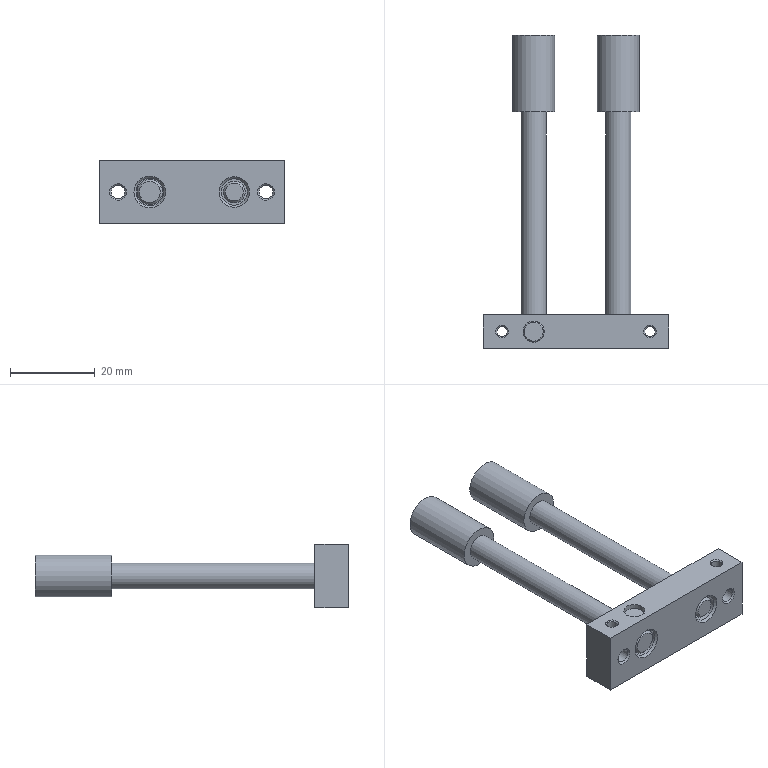Part | STEP file | ROTATION MC_NEW VER-0610_474 | 1 solid | 43 faces | box 44 x 74.1 x 15 mm | volume 10477 mm3 | plane 15 | cylinder 15 | cone 13 | commonest cylinder face diameters 2.459 x4 6 x3 3.242 x2 10 x2 5 x1 5.2 x1
STEP:
#1=CARTESIAN_POINT('',(223.531,700.368,-30.851));
#2=VERTEX_POINT('',#1);
#3=CARTESIAN_POINT('',(228.531,700.368,-30.851));
#4=DIRECTION('',(0.,1.,0.));
#5=DIRECTION('',(-1.,0.,0.));
#6=AXIS2_PLACEMENT_3D('',#3,#4,#5);
#7=CIRCLE('',#6,5.);
#8=EDGE_CURVE('',#2,#2,#7,.T.);
#9=ORIENTED_EDGE('',*,*,#8,.T.);
#10=EDGE_LOOP('',(#9));
#11=FACE_OUTER_BOUND('',#10,.T.);
#12=CARTESIAN_POINT('',(228.531,700.368,-25.851));
#13=DIRECTION('',(0.,-1.,0.));
#14=DIRECTION('',(0.,0.,-1.));
#15=AXIS2_PLACEMENT_3D('',#12,#13,#14);
#16=PLANE('',#15);
#17=ADVANCED_FACE('',(#11),#16,.F.);
#18=ORIENTED_EDGE('',*,*,#8,.F.);
#19=CARTESIAN_POINT('',(223.531,682.268,-30.851));
#20=VERTEX_POINT('',#19);
#21=CARTESIAN_POINT('',(223.531,700.368,-30.851));
#22=DIRECTION('',(0.,-1.,0.));
#23=VECTOR('',#22,5.);
#24=LINE('',#21,#23);
#25=EDGE_CURVE('',#2,#20,#24,.T.);
#26=ORIENTED_EDGE('',*,*,#25,.T.);
#27=CARTESIAN_POINT('',(228.531,682.268,-30.851));
#28=DIRECTION('',(0.,1.,0.));
#29=DIRECTION('',(-1.,0.,0.));
#30=AXIS2_PLACEMENT_3D('',#27,#28,#29);
#31=CIRCLE('',#30,5.);
#32=EDGE_CURVE('',#20,#20,#31,.T.);
#33=ORIENTED_EDGE('',*,*,#32,.T.);
#34=ORIENTED_EDGE('',*,*,#25,.F.);
#35=EDGE_LOOP('',(#18,#26,#33,#34));
#36=FACE_OUTER_BOUND('',#35,.T.);
#37=CARTESIAN_POINT('',(228.531,700.368,-30.851));
#38=DIRECTION('',(0.,1.,0.));
#39=DIRECTION('',(1.,0.,0.));
#40=AXIS2_PLACEMENT_3D('',#37,#38,#39);
#41=CYLINDRICAL_SURFACE('',#40,5.);
#42=ADVANCED_FACE('',(#36),#41,.T.);
#43=ORIENTED_EDGE('',*,*,#32,.F.);
#44=EDGE_LOOP('',(#43));
#45=FACE_OUTER_BOUND('',#44,.T.);
#46=CARTESIAN_POINT('',(225.531,682.268,-30.851));
#47=VERTEX_POINT('',#46);
#48=CARTESIAN_POINT('',(228.531,682.268,-30.851));
#49=DIRECTION('',(0.,1.,0.));
#50=DIRECTION('',(-1.,0.,0.));
#51=AXIS2_PLACEMENT_3D('',#48,#49,#50);
#52=CIRCLE('',#51,3.);
#53=EDGE_CURVE('',#47,#47,#52,.T.);
#54=ORIENTED_EDGE('',*,*,#53,.T.);
#55=EDGE_LOOP('',(#54));
#56=FACE_BOUND('',#55,.T.);
#57=CARTESIAN_POINT('',(228.531,682.268,-27.851));
#58=DIRECTION('',(0.,1.,0.));
#59=DIRECTION('',(0.,0.,1.));
#60=AXIS2_PLACEMENT_3D('',#57,#58,#59);
#61=PLANE('',#60);
#62=ADVANCED_FACE('',(#45,#56),#61,.F.);
#63=ORIENTED_EDGE('',*,*,#53,.F.);
#64=CARTESIAN_POINT('',(225.531,634.268,-30.851));
#65=VERTEX_POINT('',#64);
#66=CARTESIAN_POINT('',(225.531,700.368,-30.851));
#67=DIRECTION('',(0.,-1.,0.));
#68=VECTOR('',#67,3.);
#69=LINE('',#66,#68);
#70=EDGE_CURVE('',#47,#65,#69,.T.);
#71=ORIENTED_EDGE('',*,*,#70,.T.);
#72=CARTESIAN_POINT('',(228.531,634.268,-30.851));
#73=DIRECTION('',(0.,1.,0.));
#74=DIRECTION('',(-1.,0.,0.));
#75=AXIS2_PLACEMENT_3D('',#72,#73,#74);
#76=CIRCLE('',#75,3.);
#77=EDGE_CURVE('',#65,#65,#76,.T.);
#78=ORIENTED_EDGE('',*,*,#77,.T.);
#79=ORIENTED_EDGE('',*,*,#70,.F.);
#80=EDGE_LOOP('',(#63,#71,#78,#79));
#81=FACE_OUTER_BOUND('',#80,.T.);
#82=CARTESIAN_POINT('',(228.531,700.368,-30.851));
#83=DIRECTION('',(0.,1.,0.));
#84=DIRECTION('',(1.,0.,0.));
#85=AXIS2_PLACEMENT_3D('',#82,#83,#84);
#86=CYLINDRICAL_SURFACE('',#85,3.);
#87=ADVANCED_FACE('',(#81),#86,.T.);
#88=CARTESIAN_POINT('',(226.431,626.768,-30.851));
#89=VERTEX_POINT('',#88);
#90=CARTESIAN_POINT('',(228.531,626.768,-30.851));
#91=DIRECTION('',(0.,1.,0.));
#92=DIRECTION('',(-1.,0.,0.));
#93=AXIS2_PLACEMENT_3D('',#90,#91,#92);
#94=CIRCLE('',#93,2.1);
#95=EDGE_CURVE('',#89,#89,#94,.T.);
#96=ORIENTED_EDGE('',*,*,#95,.F.);
#97=EDGE_LOOP('',(#96));
#98=FACE_OUTER_BOUND('',#97,.T.);
#99=CARTESIAN_POINT('',(228.531,626.768,-28.751));
#100=DIRECTION('',(0.,-1.,0.));
#101=DIRECTION('',(0.,0.,-1.));
#102=AXIS2_PLACEMENT_3D('',#99,#100,#101);
#103=PLANE('',#102);
#104=ADVANCED_FACE('',(#98),#103,.T.);
#105=CARTESIAN_POINT('',(225.931,627.268,-30.851));
#106=VERTEX_POINT('',#105);
#107=CARTESIAN_POINT('',(228.531,627.268,-30.851));
#108=DIRECTION('',(0.,1.,0.));
#109=DIRECTION('',(-1.,0.,0.));
#110=AXIS2_PLACEMENT_3D('',#107,#108,#109);
#111=CIRCLE('',#110,2.6);
#112=EDGE_CURVE('',#106,#106,#111,.T.);
#113=ORIENTED_EDGE('',*,*,#112,.F.);
#114=CARTESIAN_POINT('',(225.931,627.268,-30.851));
#115=DIRECTION('',(0.7071,-0.7071,0.));
#116=VECTOR('',#115,2.6);
#117=LINE('',#114,#116);
#118=EDGE_CURVE('',#106,#89,#117,.T.);
#119=ORIENTED_EDGE('',*,*,#118,.T.);
#120=ORIENTED_EDGE('',*,*,#95,.T.);
#121=ORIENTED_EDGE('',*,*,#118,.F.);
#122=EDGE_LOOP('',(#113,#119,#120,#121));
#123=FACE_OUTER_BOUND('',#122,.T.);
#124=CARTESIAN_POINT('',(228.531,627.268,-30.851));
#125=DIRECTION('',(0.,1.,0.));
#126=DIRECTION('',(1.,0.,0.));
#127=AXIS2_PLACEMENT_3D('',#124,#125,#126);
#128=CONICAL_SURFACE('',#127,2.6,0.7854);
#129=ADVANCED_FACE('',(#123),#128,.T.);
#130=CARTESIAN_POINT('',(225.931,630.268,-30.851));
#131=VERTEX_POINT('',#130);
#132=CARTESIAN_POINT('',(228.531,630.268,-30.851));
#133=DIRECTION('',(0.,1.,0.));
#134=DIRECTION('',(-1.,0.,0.));
#135=AXIS2_PLACEMENT_3D('',#132,#133,#134);
#136=CIRCLE('',#135,2.6);
#137=EDGE_CURVE('',#131,#131,#136,.T.);
#138=ORIENTED_EDGE('',*,*,#137,.F.);
#139=CARTESIAN_POINT('',(225.931,630.268,-30.851));
#140=DIRECTION('',(0.,-1.,0.));
#141=VECTOR('',#140,2.6);
#142=LINE('',#139,#141);
#143=EDGE_CURVE('',#131,#106,#142,.T.);
#144=ORIENTED_EDGE('',*,*,#143,.T.);
#145=ORIENTED_EDGE('',*,*,#112,.T.);
#146=ORIENTED_EDGE('',*,*,#143,.F.);
#147=EDGE_LOOP('',(#138,#144,#145,#146));
#148=FACE_OUTER_BOUND('',#147,.T.);
#149=CARTESIAN_POINT('',(228.531,630.268,-30.851));
#150=DIRECTION('',(0.,1.,0.));
#151=DIRECTION('',(1.,0.,0.));
#152=AXIS2_PLACEMENT_3D('',#149,#150,#151);
#153=CYLINDRICAL_SURFACE('',#152,2.6);
#154=ADVANCED_FACE('',(#148),#153,.T.);
#155=CARTESIAN_POINT('',(225.431,630.268,-30.851));
#156=VERTEX_POINT('',#155);
#157=CARTESIAN_POINT('',(228.531,630.268,-30.851));
#158=DIRECTION('',(0.,1.,0.));
#159=DIRECTION('',(-1.,0.,0.));
#160=AXIS2_PLACEMENT_3D('',#157,#158,#159);
#161=CIRCLE('',#160,3.1);
#162=EDGE_CURVE('',#156,#156,#161,.T.);
#163=ORIENTED_EDGE('',*,*,#162,.F.);
#164=EDGE_LOOP('',(#163));
#165=FACE_OUTER_BOUND('',#164,.T.);
#166=ORIENTED_EDGE('',*,*,#137,.T.);
#167=EDGE_LOOP('',(#166));
#168=FACE_BOUND('',#167,.T.);
#169=CARTESIAN_POINT('',(228.531,630.268,-27.751));
#170=DIRECTION('',(0.,-1.,0.));
#171=DIRECTION('',(0.,0.,-1.));
#172=AXIS2_PLACEMENT_3D('',#169,#170,#171);
#173=PLANE('',#172);
#174=ADVANCED_FACE('',(#165,#168),#173,.T.);
#175=CARTESIAN_POINT('',(231.631,626.768,-30.851));
#176=VERTEX_POINT('',#175);
#177=CARTESIAN_POINT('',(225.431,626.768,-30.851));
#178=VERTEX_POINT('',#177);
#179=CARTESIAN_POINT('',(228.531,626.768,-30.851));
#180=DIRECTION('',(0.,1.,0.));
#181=DIRECTION('',(-1.,0.,0.));
#182=AXIS2_PLACEMENT_3D('',#179,#180,#181);
#183=CIRCLE('',#182,3.1);
#184=EDGE_CURVE('',#176,#178,#183,.T.);
#185=ORIENTED_EDGE('',*,*,#184,.F.);
#186=CARTESIAN_POINT('',(228.531,626.768,-30.851));
#187=DIRECTION('',(0.,1.,0.));
#188=DIRECTION('',(-1.,0.,0.));
#189=AXIS2_PLACEMENT_3D('',#186,#187,#188);
#190=CIRCLE('',#189,3.1);
#191=EDGE_CURVE('',#178,#176,#190,.T.);
#192=ORIENTED_EDGE('',*,*,#191,.F.);
#193=CARTESIAN_POINT('',(225.431,630.268,-30.851));
#194=DIRECTION('',(0.,1.,0.));
#195=VECTOR('',#194,3.1);
#196=LINE('',#193,#195);
#197=EDGE_CURVE('',#178,#156,#196,.T.);
#198=ORIENTED_EDGE('',*,*,#197,.T.);
#199=ORIENTED_EDGE('',*,*,#162,.T.);
#200=ORIENTED_EDGE('',*,*,#197,.F.);
#201=EDGE_LOOP('',(#185,#192,#198,#199,#200));
#202=FACE_OUTER_BOUND('',#201,.T.);
#203=CARTESIAN_POINT('',(228.531,630.268,-30.851));
#204=DIRECTION('',(0.,1.,0.));
#205=DIRECTION('',(1.,0.,0.));
#206=AXIS2_PLACEMENT_3D('',#203,#204,#205);
#207=CYLINDRICAL_SURFACE('',#206,3.1);
#208=ADVANCED_FACE('',(#202),#207,.F.);
#209=ORIENTED_EDGE('',*,*,#184,.T.);
#210=ORIENTED_EDGE('',*,*,#191,.T.);
#211=CARTESIAN_POINT('',(232.131,626.268,-30.851));
#212=VERTEX_POINT('',#211);
#213=CARTESIAN_POINT('',(232.131,626.268,-30.851));
#214=DIRECTION('',(0.7071,-0.7071,0.));
#215=VECTOR('',#214,3.6);
#216=LINE('',#213,#215);
#217=EDGE_CURVE('',#176,#212,#216,.T.);
#218=ORIENTED_EDGE('',*,*,#217,.T.);
#219=CARTESIAN_POINT('',(224.931,626.268,-30.851));
#220=VERTEX_POINT('',#219);
#221=CARTESIAN_POINT('',(228.531,626.268,-30.851));
#222=DIRECTION('',(0.,1.,0.));
#223=DIRECTION('',(-1.,0.,0.));
#224=AXIS2_PLACEMENT_3D('',#221,#222,#223);
#225=CIRCLE('',#224,3.6);
#226=EDGE_CURVE('',#220,#212,#225,.T.);
#227=ORIENTED_EDGE('',*,*,#226,.F.);
#228=CARTESIAN_POINT('',(228.531,626.268,-30.851));
#229=DIRECTION('',(0.,1.,0.));
#230=DIRECTION('',(-1.,0.,0.));
#231=AXIS2_PLACEMENT_3D('',#228,#229,#230);
#232=CIRCLE('',#231,3.6);
#233=EDGE_CURVE('',#212,#220,#232,.T.);
#234=ORIENTED_EDGE('',*,*,#233,.F.);
#235=ORIENTED_EDGE('',*,*,#217,.F.);
#236=EDGE_LOOP('',(#209,#210,#218,#227,#234,#235));
#237=FACE_OUTER_BOUND('',#236,.T.);
#238=CARTESIAN_POINT('',(228.531,626.268,-30.851));
#239=DIRECTION('',(0.,-1.,0.));
#240=DIRECTION('',(-1.,0.,0.));
#241=AXIS2_PLACEMENT_3D('',#238,#239,#240);
#242=CONICAL_SURFACE('',#241,3.6,0.7854);
#243=ADVANCED_FACE('',(#237),#242,.F.);
#244=CARTESIAN_POINT('',(206.281,630.268,-24.351));
#245=VERTEX_POINT('',#244);
#246=CARTESIAN_POINT('',(208.531,630.268,-24.351));
#247=DIRECTION('',(0.,0.,-1.));
#248=DIRECTION('',(-1.,0.,0.));
#249=AXIS2_PLACEMENT_3D('',#246,#247,#248);
#250=CIRCLE('',#249,2.25);
#251=EDGE_CURVE('',#245,#245,#250,.T.);
#252=ORIENTED_EDGE('',*,*,#251,.F.);
#253=EDGE_LOOP('',(#252));
#254=FACE_OUTER_BOUND('',#253,.T.);
#255=CARTESIAN_POINT('',(208.531,632.518,-24.351));
#256=DIRECTION('',(0.,0.,1.));
#257=DIRECTION('',(1.,0.,0.));
#258=AXIS2_PLACEMENT_3D('',#255,#256,#257);
#259=PLANE('',#258);
#260=ADVANCED_FACE('',(#254),#259,.T.);
#261=CARTESIAN_POINT('',(206.031,630.268,-24.601));
#262=VERTEX_POINT('',#261);
#263=CARTESIAN_POINT('',(208.531,630.268,-24.601));
#264=DIRECTION('',(0.,0.,-1.));
#265=DIRECTION('',(-1.,0.,0.));
#266=AXIS2_PLACEMENT_3D('',#263,#264,#265);
#267=CIRCLE('',#266,2.5);
#268=EDGE_CURVE('',#262,#262,#267,.T.);
#269=ORIENTED_EDGE('',*,*,#268,.F.);
#270=CARTESIAN_POINT('',(206.031,630.268,-24.601));
#271=DIRECTION('',(0.7071,0.,0.7071));
#272=VECTOR('',#271,2.5);
#273=LINE('',#270,#272);
#274=EDGE_CURVE('',#262,#245,#273,.T.);
#275=ORIENTED_EDGE('',*,*,#274,.T.);
#276=ORIENTED_EDGE('',*,*,#251,.T.);
#277=ORIENTED_EDGE('',*,*,#274,.F.);
#278=EDGE_LOOP('',(#269,#275,#276,#277));
#279=FACE_OUTER_BOUND('',#278,.T.);
#280=CARTESIAN_POINT('',(208.531,630.268,-24.601));
#281=DIRECTION('',(0.,0.,-1.));
#282=DIRECTION('',(1.,0.,0.));
#283=AXIS2_PLACEMENT_3D('',#280,#281,#282);
#284=CONICAL_SURFACE('',#283,2.5,0.7854);
#285=ADVANCED_FACE('',(#279),#284,.T.);
#286=CARTESIAN_POINT('',(206.031,630.268,-23.351));
#287=VERTEX_POINT('',#286);
#288=CARTESIAN_POINT('',(208.531,630.268,-23.351));
#289=DIRECTION('',(0.,0.,-1.));
#290=DIRECTION('',(-1.,0.,0.));
#291=AXIS2_PLACEMENT_3D('',#288,#289,#290);
#292=CIRCLE('',#291,2.5);
#293=EDGE_CURVE('',#287,#287,#292,.T.);
#294=ORIENTED_EDGE('',*,*,#293,.F.);
#295=CARTESIAN_POINT('',(206.031,630.268,-24.351));
#296=DIRECTION('',(0.,0.,-1.));
#297=VECTOR('',#296,2.5);
#298=LINE('',#295,#297);
#299=EDGE_CURVE('',#287,#262,#298,.T.);
#300=ORIENTED_EDGE('',*,*,#299,.T.);
#301=ORIENTED_EDGE('',*,*,#268,.T.);
#302=ORIENTED_EDGE('',*,*,#299,.F.);
#303=EDGE_LOOP('',(#294,#300,#301,#302));
#304=FACE_OUTER_BOUND('',#303,.T.);
#305=CARTESIAN_POINT('',(208.531,630.268,-24.351));
#306=DIRECTION('',(0.,0.,-1.));
#307=DIRECTION('',(1.,0.,0.));
#308=AXIS2_PLACEMENT_3D('',#305,#306,#307);
#309=CYLINDRICAL_SURFACE('',#308,2.5);
#310=ADVANCED_FACE('',(#304),#309,.F.);
#311=CARTESIAN_POINT('',(203.531,700.368,-30.851));
#312=VERTEX_POINT('',#311);
#313=CARTESIAN_POINT('',(208.531,700.368,-30.851));
#314=DIRECTION('',(0.,1.,0.));
#315=DIRECTION('',(-1.,0.,0.));
#316=AXIS2_PLACEMENT_3D('',#313,#314,#315);
#317=CIRCLE('',#316,5.);
#318=EDGE_CURVE('',#312,#312,#317,.T.);
#319=ORIENTED_EDGE('',*,*,#318,.T.);
#320=EDGE_LOOP('',(#319));
#321=FACE_OUTER_BOUND('',#320,.T.);
#322=CARTESIAN_POINT('',(208.531,700.368,-25.851));
#323=DIRECTION('',(0.,-1.,0.));
#324=DIRECTION('',(0.,0.,-1.));
#325=AXIS2_PLACEMENT_3D('',#322,#323,#324);
#326=PLANE('',#325);
#327=ADVANCED_FACE('',(#321),#326,.F.);
#328=ORIENTED_EDGE('',*,*,#318,.F.);
#329=CARTESIAN_POINT('',(203.531,682.268,-30.851));
#330=VERTEX_POINT('',#329);
#331=CARTESIAN_POINT('',(203.531,700.368,-30.851));
#332=DIRECTION('',(0.,-1.,0.));
#333=VECTOR('',#332,5.);
#334=LINE('',#331,#333);
#335=EDGE_CURVE('',#312,#330,#334,.T.);
#336=ORIENTED_EDGE('',*,*,#335,.T.);
#337=CARTESIAN_POINT('',(208.531,682.268,-30.851));
#338=DIRECTION('',(0.,1.,0.));
#339=DIRECTION('',(-1.,0.,0.));
#340=AXIS2_PLACEMENT_3D('',#337,#338,#339);
#341=CIRCLE('',#340,5.);
#342=EDGE_CURVE('',#330,#330,#341,.T.);
#343=ORIENTED_EDGE('',*,*,#342,.T.);
#344=ORIENTED_EDGE('',*,*,#335,.F.);
#345=EDGE_LOOP('',(#328,#336,#343,#344));
#346=FACE_OUTER_BOUND('',#345,.T.);
#347=CARTESIAN_POINT('',(208.531,700.368,-30.851));
#348=DIRECTION('',(0.,1.,0.));
#349=DIRECTION('',(1.,0.,0.));
#350=AXIS2_PLACEMENT_3D('',#347,#348,#349);
#351=CYLINDRICAL_SURFACE('',#350,5.);
#352=ADVANCED_FACE('',(#346),#351,.T.);
#353=ORIENTED_EDGE('',*,*,#342,.F.);
#354=EDGE_LOOP('',(#353));
#355=FACE_OUTER_BOUND('',#354,.T.);
#356=CARTESIAN_POINT('',(205.531,682.268,-30.851));
#357=VERTEX_POINT('',#356);
#358=CARTESIAN_POINT('',(208.531,682.268,-30.851));
#359=DIRECTION('',(0.,1.,0.));
#360=DIRECTION('',(-1.,0.,0.));
#361=AXIS2_PLACEMENT_3D('',#358,#359,#360);
#362=CIRCLE('',#361,3.);
#363=EDGE_CURVE('',#357,#357,#362,.T.);
#364=ORIENTED_EDGE('',*,*,#363,.T.);
#365=EDGE_LOOP('',(#364));
#366=FACE_BOUND('',#365,.T.);
#367=CARTESIAN_POINT('',(208.531,682.268,-27.851));
#368=DIRECTION('',(0.,1.,0.));
#369=DIRECTION('',(0.,0.,1.));
#370=AXIS2_PLACEMENT_3D('',#367,#368,#369);
#371=PLANE('',#370);
#372=ADVANCED_FACE('',(#355,#366),#371,.F.);
#373=ORIENTED_EDGE('',*,*,#363,.F.);
#374=CARTESIAN_POINT('',(205.531,634.268,-30.851));
#375=VERTEX_POINT('',#374);
#376=CARTESIAN_POINT('',(205.531,700.368,-30.851));
#377=DIRECTION('',(0.,-1.,0.));
#378=VECTOR('',#377,3.);
#379=LINE('',#376,#378);
#380=EDGE_CURVE('',#357,#375,#379,.T.);
#381=ORIENTED_EDGE('',*,*,#380,.T.);
#382=CARTESIAN_POINT('',(208.531,634.268,-30.851));
#383=DIRECTION('',(0.,1.,0.));
#384=DIRECTION('',(-1.,0.,0.));
#385=AXIS2_PLACEMENT_3D('',#382,#383,#384);
#386=CIRCLE('',#385,3.);
#387=EDGE_CURVE('',#375,#375,#386,.T.);
#388=ORIENTED_EDGE('',*,*,#387,.T.);
#389=ORIENTED_EDGE('',*,*,#380,.F.);
#390=EDGE_LOOP('',(#373,#381,#388,#389));
#391=FACE_OUTER_BOUND('',#390,.T.);
#392=CARTESIAN_POINT('',(208.531,700.368,-30.851));
#393=DIRECTION('',(0.,1.,0.));
#394=DIRECTION('',(1.,0.,0.));
#395=AXIS2_PLACEMENT_3D('',#392,#393,#394);
#396=CYLINDRICAL_SURFACE('',#395,3.);
#397=ADVANCED_FACE('',(#391),#396,.T.);
#398=CARTESIAN_POINT('',(206.031,626.768,-30.851));
#399=VERTEX_POINT('',#398);
#400=CARTESIAN_POINT('',(208.531,626.768,-30.851));
#401=DIRECTION('',(0.,1.,0.));
#402=DIRECTION('',(-1.,0.,0.));
#403=AXIS2_PLACEMENT_3D('',#400,#401,#402);
#404=CIRCLE('',#403,2.5);
#405=EDGE_CURVE('',#399,#399,#404,.T.);
#406=ORIENTED_EDGE('',*,*,#405,.F.);
#407=EDGE_LOOP('',(#406));
#408=FACE_OUTER_BOUND('',#407,.T.);
#409=CARTESIAN_POINT('',(208.531,626.768,-28.351));
#410=DIRECTION('',(0.,-1.,0.));
#411=DIRECTION('',(0.,0.,-1.));
#412=AXIS2_PLACEMENT_3D('',#409,#410,#411);
#413=PLANE('',#412);
#414=ADVANCED_FACE('',(#408),#413,.T.);
#415=CARTESIAN_POINT('',(205.531,627.268,-30.851));
#416=VERTEX_POINT('',#415);
#417=CARTESIAN_POINT('',(208.531,627.268,-30.851));
#418=DIRECTION('',(0.,1.,0.));
#419=DIRECTION('',(-1.,0.,0.));
#420=AXIS2_PLACEMENT_3D('',#417,#418,#419);
#421=CIRCLE('',#420,3.);
#422=EDGE_CURVE('',#416,#416,#421,.T.);
#423=ORIENTED_EDGE('',*,*,#422,.F.);
#424=CARTESIAN_POINT('',(205.531,627.268,-30.851));
#425=DIRECTION('',(0.7071,-0.7071,0.));
#426=VECTOR('',#425,3.);
#427=LINE('',#424,#426);
#428=EDGE_CURVE('',#416,#399,#427,.T.);
#429=ORIENTED_EDGE('',*,*,#428,.T.);
#430=ORIENTED_EDGE('',*,*,#405,.T.);
#431=ORIENTED_EDGE('',*,*,#428,.F.);
#432=EDGE_LOOP('',(#423,#429,#430,#431));
#433=FACE_OUTER_BOUND('',#432,.T.);
#434=CARTESIAN_POINT('',(208.531,627.268,-30.851));
#435=DIRECTION('',(0.,1.,0.));
#436=DIRECTION('',(1.,0.,0.));
#437=AXIS2_PLACEMENT_3D('',#434,#435,#436);
#438=CONICAL_SURFACE('',#437,3.,0.7854);
#439=ADVANCED_FACE('',(#433),#438,.T.);
#440=CARTESIAN_POINT('',(205.531,630.268,-30.851));
#441=VERTEX_POINT('',#440);
#442=CARTESIAN_POINT('',(208.531,630.268,-30.851));
#443=DIRECTION('',(0.,1.,0.));
#444=DIRECTION('',(-1.,0.,0.));
#445=AXIS2_PLACEMENT_3D('',#442,#443,#444);
#446=CIRCLE('',#445,3.);
#447=EDGE_CURVE('',#441,#441,#446,.T.);
#448=ORIENTED_EDGE('',*,*,#447,.F.);
#449=CARTESIAN_POINT('',(205.531,630.268,-30.851));
#450=DIRECTION('',(0.,-1.,0.));
#451=VECTOR('',#450,3.);
#452=LINE('',#449,#451);
#453=EDGE_CURVE('',#441,#416,#452,.T.);
#454=ORIENTED_EDGE('',*,*,#453,.T.);
#455=ORIENTED_EDGE('',*,*,#422,.T.);
#456=ORIENTED_EDGE('',*,*,#453,.F.);
#457=EDGE_LOOP('',(#448,#454,#455,#456));
#458=FACE_OUTER_BOUND('',#457,.T.);
#459=CARTESIAN_POINT('',(208.531,630.268,-30.851));
#460=DIRECTION('',(0.,1.,0.));
#461=DIRECTION('',(1.,0.,0.));
#462=AXIS2_PLACEMENT_3D('',#459,#460,#461);
#463=CYLINDRICAL_SURFACE('',#462,3.);
#464=ADVANCED_FACE('',(#458),#463,.T.);
#465=CARTESIAN_POINT('',(205.281,630.268,-30.851));
#466=VERTEX_POINT('',#465);
#467=CARTESIAN_POINT('',(208.531,630.268,-30.851));
#468=DIRECTION('',(0.,1.,0.));
#469=DIRECTION('',(-1.,0.,0.));
#470=AXIS2_PLACEMENT_3D('',#467,#468,#469);
#471=CIRCLE('',#470,3.25);
#472=EDGE_CURVE('',#466,#466,#471,.T.);
#473=ORIENTED_EDGE('',*,*,#472,.F.);
#474=EDGE_LOOP('',(#473));
#475=FACE_OUTER_BOUND('',#474,.T.);
#476=ORIENTED_EDGE('',*,*,#447,.T.);
#477=EDGE_LOOP('',(#476));
#478=FACE_BOUND('',#477,.T.);
#479=CARTESIAN_POINT('',(208.531,630.268,-27.601));
#480=DIRECTION('',(0.,-1.,0.));
#481=DIRECTION('',(0.,0.,-1.));
#482=AXIS2_PLACEMENT_3D('',#479,#480,#481);
#483=PLANE('',#482);
#484=ADVANCED_FACE('',(#475,#478),#483,.T.);
#485=CARTESIAN_POINT('',(211.781,626.768,-30.851));
#486=VERTEX_POINT('',#485);
#487=CARTESIAN_POINT('',(205.281,626.768,-30.851));
#488=VERTEX_POINT('',#487);
#489=CARTESIAN_POINT('',(208.531,626.768,-30.851));
#490=DIRECTION('',(0.,1.,0.));
#491=DIRECTION('',(-1.,0.,0.));
#492=AXIS2_PLACEMENT_3D('',#489,#490,#491);
#493=CIRCLE('',#492,3.25);
#494=EDGE_CURVE('',#486,#488,#493,.T.);
#495=ORIENTED_EDGE('',*,*,#494,.F.);
#496=CARTESIAN_POINT('',(208.531,626.768,-30.851));
#497=DIRECTION('',(0.,1.,0.));
#498=DIRECTION('',(-1.,0.,0.));
#499=AXIS2_PLACEMENT_3D('',#496,#497,#498);
#500=CIRCLE('',#499,3.25);
#501=EDGE_CURVE('',#488,#486,#500,.T.);
#502=ORIENTED_EDGE('',*,*,#501,.F.);
#503=CARTESIAN_POINT('',(205.281,630.268,-30.851));
#504=DIRECTION('',(0.,1.,0.));
#505=VECTOR('',#504,3.25);
#506=LINE('',#503,#505);
#507=EDGE_CURVE('',#488,#466,#506,.T.);
#508=ORIENTED_EDGE('',*,*,#507,.T.);
#509=ORIENTED_EDGE('',*,*,#472,.T.);
#510=ORIENTED_EDGE('',*,*,#507,.F.);
#511=EDGE_LOOP('',(#495,#502,#508,#509,#510));
#512=FACE_OUTER_BOUND('',#511,.T.);
#513=CARTESIAN_POINT('',(208.531,630.268,-30.851));
#514=DIRECTION('',(0.,1.,0.));
#515=DIRECTION('',(1.,0.,0.));
#516=AXIS2_PLACEMENT_3D('',#513,#514,#515);
#517=CYLINDRICAL_SURFACE('',#516,3.25);
#518=ADVANCED_FACE('',(#512),#517,.F.);
#519=ORIENTED_EDGE('',*,*,#494,.T.);
#520=ORIENTED_EDGE('',*,*,#501,.T.);
#521=CARTESIAN_POINT('',(212.281,626.268,-30.851));
#522=VERTEX_POINT('',#521);
#523=CARTESIAN_POINT('',(212.281,626.268,-30.851));
#524=DIRECTION('',(0.7071,-0.7071,0.));
#525=VECTOR('',#524,3.75);
#526=LINE('',#523,#525);
#527=EDGE_CURVE('',#486,#522,#526,.T.);
#528=ORIENTED_EDGE('',*,*,#527,.T.);
#529=CARTESIAN_POINT('',(204.781,626.268,-30.851));
#530=VERTEX_POINT('',#529);
#531=CARTESIAN_POINT('',(208.531,626.268,-30.851));
#532=DIRECTION('',(0.,1.,0.));
#533=DIRECTION('',(-1.,0.,0.));
#534=AXIS2_PLACEMENT_3D('',#531,#532,#533);
#535=CIRCLE('',#534,3.75);
#536=EDGE_CURVE('',#530,#522,#535,.T.);
#537=ORIENTED_EDGE('',*,*,#536,.F.);
#538=CARTESIAN_POINT('',(208.531,626.268,-30.851));
#539=DIRECTION('',(0.,1.,0.));
#540=DIRECTION('',(-1.,0.,0.));
#541=AXIS2_PLACEMENT_3D('',#538,#539,#540);
#542=CIRCLE('',#541,3.75);
#543=EDGE_CURVE('',#522,#530,#542,.T.);
#544=ORIENTED_EDGE('',*,*,#543,.F.);
#545=ORIENTED_EDGE('',*,*,#527,.F.);
#546=EDGE_LOOP('',(#519,#520,#528,#537,#544,#545));
#547=FACE_OUTER_BOUND('',#546,.T.);
#548=CARTESIAN_POINT('',(208.531,626.268,-30.851));
#549=DIRECTION('',(0.,-1.,0.));
#550=DIRECTION('',(-1.,0.,0.));
#551=AXIS2_PLACEMENT_3D('',#548,#549,#550);
#552=CONICAL_SURFACE('',#551,3.75,0.7854);
#553=ADVANCED_FACE('',(#547),#552,.F.);
#554=CARTESIAN_POINT('',(199.801,630.268,-23.622));
#555=VERTEX_POINT('',#554);
#556=CARTESIAN_POINT('',(202.26,630.268,-23.622));
#557=VERTEX_POINT('',#556);
#558=CARTESIAN_POINT('',(201.031,630.268,-23.622));
#559=DIRECTION('',(0.,0.,-1.));
#560=DIRECTION('',(-1.,0.,0.));
#561=AXIS2_PLACEMENT_3D('',#558,#559,#560);
#562=CIRCLE('',#561,1.23);
#563=EDGE_CURVE('',#555,#557,#562,.T.);
#564=ORIENTED_EDGE('',*,*,#563,.T.);
#565=CARTESIAN_POINT('',(202.531,630.268,-23.351));
#566=VERTEX_POINT('',#565);
#567=CARTESIAN_POINT('',(202.531,630.268,-23.351));
#568=DIRECTION('',(0.7071,0.,0.7071));
#569=VECTOR('',#568,1.5);
#570=LINE('',#567,#569);
#571=EDGE_CURVE('',#557,#566,#570,.T.);
#572=ORIENTED_EDGE('',*,*,#571,.T.);
#573=CARTESIAN_POINT('',(199.531,630.268,-23.351));
#574=VERTEX_POINT('',#573);
#575=CARTESIAN_POINT('',(201.031,630.268,-23.351));
#576=DIRECTION('',(0.,0.,-1.));
#577=DIRECTION('',(-1.,0.,0.));
#578=AXIS2_PLACEMENT_3D('',#575,#576,#577);
#579=CIRCLE('',#578,1.5);
#580=EDGE_CURVE('',#574,#566,#579,.T.);
#581=ORIENTED_EDGE('',*,*,#580,.F.);
#582=CARTESIAN_POINT('',(201.031,630.268,-23.351));
#583=DIRECTION('',(0.,0.,-1.));
#584=DIRECTION('',(-1.,0.,0.));
#585=AXIS2_PLACEMENT_3D('',#582,#583,#584);
#586=CIRCLE('',#585,1.5);
#587=EDGE_CURVE('',#566,#574,#586,.T.);
#588=ORIENTED_EDGE('',*,*,#587,.F.);
#589=ORIENTED_EDGE('',*,*,#571,.F.);
#590=CARTESIAN_POINT('',(201.031,630.268,-23.622));
#591=DIRECTION('',(0.,0.,-1.));
#592=DIRECTION('',(-1.,0.,0.));
#593=AXIS2_PLACEMENT_3D('',#590,#591,#592);
#594=CIRCLE('',#593,1.23);
#595=EDGE_CURVE('',#557,#555,#594,.T.);
#596=ORIENTED_EDGE('',*,*,#595,.T.);
#597=EDGE_LOOP('',(#564,#572,#581,#588,#589,#596));
#598=FACE_OUTER_BOUND('',#597,.T.);
#599=CARTESIAN_POINT('',(201.031,630.268,-23.351));
#600=DIRECTION('',(0.,0.,1.));
#601=DIRECTION('',(-1.,0.,0.));
#602=AXIS2_PLACEMENT_3D('',#599,#600,#601);
#603=CONICAL_SURFACE('',#602,1.5,0.7854);
#604=ADVANCED_FACE('',(#598),#603,.F.);
#605=ORIENTED_EDGE('',*,*,#563,.F.);
#606=CARTESIAN_POINT('',(199.801,630.268,-29.795));
#607=VERTEX_POINT('',#606);
#608=CARTESIAN_POINT('',(199.801,630.268,-38.351));
#609=DIRECTION('',(0.,0.,-1.));
#610=VECTOR('',#609,1.23);
#611=LINE('',#608,#610);
#612=EDGE_CURVE('',#555,#607,#611,.T.);
#613=ORIENTED_EDGE('',*,*,#612,.T.);
#614=CARTESIAN_POINT('',(199.801,630.268,-29.795));
#615=CARTESIAN_POINT('',(199.801,630.186,-29.795));
#616=CARTESIAN_POINT('',(199.81,630.103,-29.785));
#617=CARTESIAN_POINT('',(199.843,629.941,-29.748));
#618=CARTESIAN_POINT('',(199.867,629.863,-29.722));
#619=CARTESIAN_POINT('',(199.962,629.639,-29.629));
#620=CARTESIAN_POINT('',(200.055,629.506,-29.551));
#621=CARTESIAN_POINT('',(200.266,629.295,-29.417));
#622=CARTESIAN_POINT('',(200.399,629.201,-29.35));
#623=CARTESIAN_POINT('',(200.701,629.073,-29.256));
#624=CARTESIAN_POINT('',(200.869,629.039,-29.23));
#625=CARTESIAN_POINT('',(201.193,629.039,-29.23));
#626=CARTESIAN_POINT('',(201.361,629.073,-29.256));
#627=CARTESIAN_POINT('',(201.662,629.201,-29.35));
#628=CARTESIAN_POINT('',(201.796,629.295,-29.417));
#629=CARTESIAN_POINT('',(202.007,629.506,-29.551));
#630=CARTESIAN_POINT('',(202.099,629.639,-29.629));
#631=CARTESIAN_POINT('',(202.194,629.863,-29.722));
#632=CARTESIAN_POINT('',(202.219,629.941,-29.748));
#633=CARTESIAN_POINT('',(202.252,630.103,-29.785));
#634=CARTESIAN_POINT('',(202.26,630.186,-29.795));
#635=CARTESIAN_POINT('',(202.26,630.351,-29.795));
#636=CARTESIAN_POINT('',(202.252,630.434,-29.785));
#637=CARTESIAN_POINT('',(202.219,630.596,-29.748));
#638=CARTESIAN_POINT('',(202.194,630.674,-29.722));
#639=CARTESIAN_POINT('',(202.099,630.898,-29.629));
#640=CARTESIAN_POINT('',(202.007,631.031,-29.551));
#641=CARTESIAN_POINT('',(201.796,631.242,-29.417));
#642=CARTESIAN_POINT('',(201.662,631.336,-29.35));
#643=CARTESIAN_POINT('',(201.361,631.464,-29.256));
#644=CARTESIAN_POINT('',(201.193,631.498,-29.23));
#645=CARTESIAN_POINT('',(200.869,631.498,-29.23));
#646=CARTESIAN_POINT('',(200.701,631.464,-29.256));
#647=CARTESIAN_POINT('',(200.399,631.336,-29.35));
#648=CARTESIAN_POINT('',(200.266,631.242,-29.417));
#649=CARTESIAN_POINT('',(200.055,631.031,-29.551));
#650=CARTESIAN_POINT('',(199.962,630.898,-29.629));
#651=CARTESIAN_POINT('',(199.867,630.674,-29.722));
#652=CARTESIAN_POINT('',(199.843,630.596,-29.748));
#653=CARTESIAN_POINT('',(199.81,630.434,-29.785));
#654=CARTESIAN_POINT('',(199.801,630.351,-29.795));
#655=CARTESIAN_POINT('',(199.801,630.268,-29.795));
#656=B_SPLINE_CURVE_WITH_KNOTS('',3,(#614,#615,#616,#617,#618,#619,#620,#621,#622,#623,#624,#625,#626,#627,#628,#629,#630,#631,#632,#633,#634,#635,#636,#637,#638,#639,#640,#641,#642,#643,#644,#645,#646,#647,#648,#649,#650,#651,#652,#653,#654,#655),.UNSPECIFIED.,.T.,.F.,(4,2,2,2,2,2,2,2,2,2,2,2,2,2,2,2,2,2,2,2,4),(-0.7858,-0.7609,-0.7361,-0.6864,-0.6379,-0.5893,-0.5408,-0.4922,-0.4426,-0.4177,-0.3929,-0.3681,-0.3432,-0.2935,-0.245,-0.1964,-0.1479,-0.09934,-0.04967,-0.02483,0.),.UNSPECIFIED.);
#657=EDGE_CURVE('',#607,#607,#656,.T.);
#658=ORIENTED_EDGE('',*,*,#657,.F.);
#659=ORIENTED_EDGE('',*,*,#612,.F.);
#660=ORIENTED_EDGE('',*,*,#595,.F.);
#661=EDGE_LOOP('',(#605,#613,#658,#659,#660));
#662=FACE_OUTER_BOUND('',#661,.T.);
#663=CARTESIAN_POINT('',(201.031,630.268,-38.351));
#664=DIRECTION('',(0.,0.,-1.));
#665=DIRECTION('',(1.,0.,0.));
#666=AXIS2_PLACEMENT_3D('',#663,#664,#665);
#667=CYLINDRICAL_SURFACE('',#666,1.23);
#668=ADVANCED_FACE('',(#662),#667,.F.);
#669=CARTESIAN_POINT('',(199.801,630.268,-38.081));
#670=VERTEX_POINT('',#669);
#671=CARTESIAN_POINT('',(201.031,630.268,-38.081));
#672=DIRECTION('',(0.,0.,-1.));
#673=DIRECTION('',(-1.,0.,0.));
#674=AXIS2_PLACEMENT_3D('',#671,#672,#673);
#675=CIRCLE('',#674,1.23);
#676=EDGE_CURVE('',#670,#670,#675,.T.);
#677=ORIENTED_EDGE('',*,*,#676,.F.);
#678=CARTESIAN_POINT('',(199.531,630.268,-38.351));
#679=VERTEX_POINT('',#678);
#680=CARTESIAN_POINT('',(199.801,630.268,-38.081));
#681=DIRECTION('',(-0.7071,0.,-0.7071));
#682=VECTOR('',#681,1.23);
#683=LINE('',#680,#682);
#684=EDGE_CURVE('',#670,#679,#683,.T.);
#685=ORIENTED_EDGE('',*,*,#684,.T.);
#686=CARTESIAN_POINT('',(201.031,630.268,-38.351));
#687=DIRECTION('',(0.,0.,-1.));
#688=DIRECTION('',(-1.,0.,0.));
#689=AXIS2_PLACEMENT_3D('',#686,#687,#688);
#690=CIRCLE('',#689,1.5);
#691=EDGE_CURVE('',#679,#679,#690,.T.);
#692=ORIENTED_EDGE('',*,*,#691,.T.);
#693=ORIENTED_EDGE('',*,*,#684,.F.);
#694=EDGE_LOOP('',(#677,#685,#692,#693));
#695=FACE_OUTER_BOUND('',#694,.T.);
#696=CARTESIAN_POINT('',(201.031,630.268,-38.081));
#697=DIRECTION('',(0.,0.,-1.));
#698=DIRECTION('',(1.,0.,0.));
#699=AXIS2_PLACEMENT_3D('',#696,#697,#698);
#700=CONICAL_SURFACE('',#699,1.23,0.7854);
#701=ADVANCED_FACE('',(#695),#700,.F.);
#702=CARTESIAN_POINT('',(199.801,630.268,-31.908));
#703=VERTEX_POINT('',#702);
#704=CARTESIAN_POINT('',(199.801,630.268,-31.908));
#705=CARTESIAN_POINT('',(199.801,630.351,-31.908));
#706=CARTESIAN_POINT('',(199.81,630.434,-31.918));
#707=CARTESIAN_POINT('',(199.843,630.596,-31.954));
#708=CARTESIAN_POINT('',(199.867,630.674,-31.981));
#709=CARTESIAN_POINT('',(199.962,630.898,-32.073));
#710=CARTESIAN_POINT('',(200.055,631.031,-32.152));
#711=CARTESIAN_POINT('',(200.266,631.242,-32.286));
#712=CARTESIAN_POINT('',(200.399,631.336,-32.353));
#713=CARTESIAN_POINT('',(200.701,631.464,-32.446));
#714=CARTESIAN_POINT('',(200.869,631.498,-32.472));
#715=CARTESIAN_POINT('',(201.193,631.498,-32.472));
#716=CARTESIAN_POINT('',(201.361,631.464,-32.446));
#717=CARTESIAN_POINT('',(201.662,631.336,-32.353));
#718=CARTESIAN_POINT('',(201.796,631.242,-32.286));
#719=CARTESIAN_POINT('',(202.007,631.031,-32.152));
#720=CARTESIAN_POINT('',(202.099,630.898,-32.073));
#721=CARTESIAN_POINT('',(202.194,630.674,-31.981));
#722=CARTESIAN_POINT('',(202.219,630.596,-31.954));
#723=CARTESIAN_POINT('',(202.252,630.434,-31.918));
#724=CARTESIAN_POINT('',(202.26,630.351,-31.908));
#725=CARTESIAN_POINT('',(202.26,630.186,-31.908));
#726=CARTESIAN_POINT('',(202.252,630.103,-31.918));
#727=CARTESIAN_POINT('',(202.219,629.941,-31.954));
#728=CARTESIAN_POINT('',(202.194,629.863,-31.981));
#729=CARTESIAN_POINT('',(202.099,629.639,-32.073));
#730=CARTESIAN_POINT('',(202.007,629.506,-32.152));
#731=CARTESIAN_POINT('',(201.796,629.295,-32.286));
#732=CARTESIAN_POINT('',(201.662,629.201,-32.353));
#733=CARTESIAN_POINT('',(201.361,629.073,-32.446));
#734=CARTESIAN_POINT('',(201.193,629.039,-32.472));
#735=CARTESIAN_POINT('',(200.869,629.039,-32.472));
#736=CARTESIAN_POINT('',(200.701,629.073,-32.446));
#737=CARTESIAN_POINT('',(200.399,629.201,-32.353));
#738=CARTESIAN_POINT('',(200.266,629.295,-32.286));
#739=CARTESIAN_POINT('',(200.055,629.506,-32.152));
#740=CARTESIAN_POINT('',(199.962,629.639,-32.073));
#741=CARTESIAN_POINT('',(199.867,629.863,-31.981));
#742=CARTESIAN_POINT('',(199.843,629.941,-31.954));
#743=CARTESIAN_POINT('',(199.81,630.103,-31.918));
#744=CARTESIAN_POINT('',(199.801,630.186,-31.908));
#745=CARTESIAN_POINT('',(199.801,630.268,-31.908));
#746=B_SPLINE_CURVE_WITH_KNOTS('',3,(#704,#705,#706,#707,#708,#709,#710,#711,#712,#713,#714,#715,#716,#717,#718,#719,#720,#721,#722,#723,#724,#725,#726,#727,#728,#729,#730,#731,#732,#733,#734,#735,#736,#737,#738,#739,#740,#741,#742,#743,#744,#745),.UNSPECIFIED.,.T.,.F.,(4,2,2,2,2,2,2,2,2,2,2,2,2,2,2,2,2,2,2,2,4),(-0.7858,-0.7609,-0.7361,-0.6864,-0.6379,-0.5893,-0.5408,-0.4922,-0.4426,-0.4177,-0.3929,-0.3681,-0.3432,-0.2935,-0.245,-0.1964,-0.1479,-0.09934,-0.04967,-0.02483,0.),.UNSPECIFIED.);
#747=EDGE_CURVE('',#703,#703,#746,.T.);
#748=ORIENTED_EDGE('',*,*,#747,.F.);
#749=CARTESIAN_POINT('',(199.801,630.268,-38.351));
#750=DIRECTION('',(0.,0.,-1.));
#751=VECTOR('',#750,1.23);
#752=LINE('',#749,#751);
#753=EDGE_CURVE('',#703,#670,#752,.T.);
#754=ORIENTED_EDGE('',*,*,#753,.T.);
#755=ORIENTED_EDGE('',*,*,#676,.T.);
#756=ORIENTED_EDGE('',*,*,#753,.F.);
#757=EDGE_LOOP('',(#748,#754,#755,#756));
#758=FACE_OUTER_BOUND('',#757,.T.);
#759=CARTESIAN_POINT('',(201.031,630.268,-38.351));
#760=DIRECTION('',(0.,0.,-1.));
#761=DIRECTION('',(1.,0.,0.));
#762=AXIS2_PLACEMENT_3D('',#759,#760,#761);
#763=CYLINDRICAL_SURFACE('',#762,1.23);
#764=ADVANCED_FACE('',(#758),#763,.F.);
#765=CARTESIAN_POINT('',(234.801,630.268,-23.622));
#766=VERTEX_POINT('',#765);
#767=CARTESIAN_POINT('',(237.26,630.268,-23.622));
#768=VERTEX_POINT('',#767);
#769=CARTESIAN_POINT('',(236.031,630.268,-23.622));
#770=DIRECTION('',(0.,0.,-1.));
#771=DIRECTION('',(-1.,0.,0.));
#772=AXIS2_PLACEMENT_3D('',#769,#770,#771);
#773=CIRCLE('',#772,1.23);
#774=EDGE_CURVE('',#766,#768,#773,.T.);
#775=ORIENTED_EDGE('',*,*,#774,.T.);
#776=CARTESIAN_POINT('',(237.531,630.268,-23.351));
#777=VERTEX_POINT('',#776);
#778=CARTESIAN_POINT('',(237.531,630.268,-23.351));
#779=DIRECTION('',(0.7071,0.,0.7071));
#780=VECTOR('',#779,1.5);
#781=LINE('',#778,#780);
#782=EDGE_CURVE('',#768,#777,#781,.T.);
#783=ORIENTED_EDGE('',*,*,#782,.T.);
#784=CARTESIAN_POINT('',(234.531,630.268,-23.351));
#785=VERTEX_POINT('',#784);
#786=CARTESIAN_POINT('',(236.031,630.268,-23.351));
#787=DIRECTION('',(0.,0.,-1.));
#788=DIRECTION('',(-1.,0.,0.));
#789=AXIS2_PLACEMENT_3D('',#786,#787,#788);
#790=CIRCLE('',#789,1.5);
#791=EDGE_CURVE('',#785,#777,#790,.T.);
#792=ORIENTED_EDGE('',*,*,#791,.F.);
#793=CARTESIAN_POINT('',(236.031,630.268,-23.351));
#794=DIRECTION('',(0.,0.,-1.));
#795=DIRECTION('',(-1.,0.,0.));
#796=AXIS2_PLACEMENT_3D('',#793,#794,#795);
#797=CIRCLE('',#796,1.5);
#798=EDGE_CURVE('',#777,#785,#797,.T.);
#799=ORIENTED_EDGE('',*,*,#798,.F.);
#800=ORIENTED_EDGE('',*,*,#782,.F.);
#801=CARTESIAN_POINT('',(236.031,630.268,-23.622));
#802=DIRECTION('',(0.,0.,-1.));
#803=DIRECTION('',(-1.,0.,0.));
#804=AXIS2_PLACEMENT_3D('',#801,#802,#803);
#805=CIRCLE('',#804,1.23);
#806=EDGE_CURVE('',#768,#766,#805,.T.);
#807=ORIENTED_EDGE('',*,*,#806,.T.);
#808=EDGE_LOOP('',(#775,#783,#792,#799,#800,#807));
#809=FACE_OUTER_BOUND('',#808,.T.);
#810=CARTESIAN_POINT('',(236.031,630.268,-23.351));
#811=DIRECTION('',(0.,0.,1.));
#812=DIRECTION('',(-1.,0.,0.));
#813=AXIS2_PLACEMENT_3D('',#810,#811,#812);
#814=CONICAL_SURFACE('',#813,1.5,0.7854);
#815=ADVANCED_FACE('',(#809),#814,.F.);
#816=ORIENTED_EDGE('',*,*,#774,.F.);
#817=CARTESIAN_POINT('',(234.801,630.268,-29.795));
#818=VERTEX_POINT('',#817);
#819=CARTESIAN_POINT('',(234.801,630.268,-38.351));
#820=DIRECTION('',(0.,0.,-1.));
#821=VECTOR('',#820,1.23);
#822=LINE('',#819,#821);
#823=EDGE_CURVE('',#766,#818,#822,.T.);
#824=ORIENTED_EDGE('',*,*,#823,.T.);
#825=CARTESIAN_POINT('',(234.801,630.268,-29.795));
#826=CARTESIAN_POINT('',(234.801,630.186,-29.795));
#827=CARTESIAN_POINT('',(234.81,630.103,-29.785));
#828=CARTESIAN_POINT('',(234.843,629.941,-29.748));
#829=CARTESIAN_POINT('',(234.867,629.863,-29.722));
#830=CARTESIAN_POINT('',(234.962,629.639,-29.629));
#831=CARTESIAN_POINT('',(235.055,629.506,-29.551));
#832=CARTESIAN_POINT('',(235.266,629.295,-29.417));
#833=CARTESIAN_POINT('',(235.399,629.201,-29.35));
#834=CARTESIAN_POINT('',(235.701,629.073,-29.256));
#835=CARTESIAN_POINT('',(235.869,629.039,-29.23));
#836=CARTESIAN_POINT('',(236.193,629.039,-29.23));
#837=CARTESIAN_POINT('',(236.361,629.073,-29.256));
#838=CARTESIAN_POINT('',(236.662,629.201,-29.35));
#839=CARTESIAN_POINT('',(236.796,629.295,-29.417));
#840=CARTESIAN_POINT('',(237.007,629.506,-29.551));
#841=CARTESIAN_POINT('',(237.099,629.639,-29.629));
#842=CARTESIAN_POINT('',(237.194,629.863,-29.722));
#843=CARTESIAN_POINT('',(237.219,629.941,-29.748));
#844=CARTESIAN_POINT('',(237.252,630.103,-29.785));
#845=CARTESIAN_POINT('',(237.26,630.186,-29.795));
#846=CARTESIAN_POINT('',(237.26,630.351,-29.795));
#847=CARTESIAN_POINT('',(237.252,630.434,-29.785));
#848=CARTESIAN_POINT('',(237.219,630.596,-29.748));
#849=CARTESIAN_POINT('',(237.194,630.674,-29.722));
#850=CARTESIAN_POINT('',(237.099,630.898,-29.629));
#851=CARTESIAN_POINT('',(237.007,631.031,-29.551));
#852=CARTESIAN_POINT('',(236.796,631.242,-29.417));
#853=CARTESIAN_POINT('',(236.662,631.336,-29.35));
#854=CARTESIAN_POINT('',(236.361,631.464,-29.256));
#855=CARTESIAN_POINT('',(236.193,631.498,-29.23));
#856=CARTESIAN_POINT('',(235.869,631.498,-29.23));
#857=CARTESIAN_POINT('',(235.701,631.464,-29.256));
#858=CARTESIAN_POINT('',(235.399,631.336,-29.35));
#859=CARTESIAN_POINT('',(235.266,631.242,-29.417));
#860=CARTESIAN_POINT('',(235.055,631.031,-29.551));
#861=CARTESIAN_POINT('',(234.962,630.898,-29.629));
#862=CARTESIAN_POINT('',(234.867,630.674,-29.722));
#863=CARTESIAN_POINT('',(234.843,630.596,-29.748));
#864=CARTESIAN_POINT('',(234.81,630.434,-29.785));
#865=CARTESIAN_POINT('',(234.801,630.351,-29.795));
#866=CARTESIAN_POINT('',(234.801,630.268,-29.795));
#867=B_SPLINE_CURVE_WITH_KNOTS('',3,(#825,#826,#827,#828,#829,#830,#831,#832,#833,#834,#835,#836,#837,#838,#839,#840,#841,#842,#843,#844,#845,#846,#847,#848,#849,#850,#851,#852,#853,#854,#855,#856,#857,#858,#859,#860,#861,#862,#863,#864,#865,#866),.UNSPECIFIED.,.T.,.F.,(4,2,2,2,2,2,2,2,2,2,2,2,2,2,2,2,2,2,2,2,4),(-0.7858,-0.7609,-0.7361,-0.6864,-0.6379,-0.5893,-0.5408,-0.4922,-0.4426,-0.4177,-0.3929,-0.3681,-0.3432,-0.2935,-0.245,-0.1964,-0.1479,-0.09934,-0.04967,-0.02483,0.),.UNSPECIFIED.);
#868=EDGE_CURVE('',#818,#818,#867,.T.);
#869=ORIENTED_EDGE('',*,*,#868,.F.);
#870=ORIENTED_EDGE('',*,*,#823,.F.);
#871=ORIENTED_EDGE('',*,*,#806,.F.);
#872=EDGE_LOOP('',(#816,#824,#869,#870,#871));
#873=FACE_OUTER_BOUND('',#872,.T.);
#874=CARTESIAN_POINT('',(236.031,630.268,-38.351));
#875=DIRECTION('',(0.,0.,-1.));
#876=DIRECTION('',(1.,0.,0.));
#877=AXIS2_PLACEMENT_3D('',#874,#875,#876);
#878=CYLINDRICAL_SURFACE('',#877,1.23);
#879=ADVANCED_FACE('',(#873),#878,.F.);
#880=CARTESIAN_POINT('',(234.801,630.268,-38.081));
#881=VERTEX_POINT('',#880);
#882=CARTESIAN_POINT('',(236.031,630.268,-38.081));
#883=DIRECTION('',(0.,0.,-1.));
#884=DIRECTION('',(-1.,0.,0.));
#885=AXIS2_PLACEMENT_3D('',#882,#883,#884);
#886=CIRCLE('',#885,1.23);
#887=EDGE_CURVE('',#881,#881,#886,.T.);
#888=ORIENTED_EDGE('',*,*,#887,.F.);
#889=CARTESIAN_POINT('',(234.531,630.268,-38.351));
#890=VERTEX_POINT('',#889);
#891=CARTESIAN_POINT('',(234.801,630.268,-38.081));
#892=DIRECTION('',(-0.7071,0.,-0.7071));
#893=VECTOR('',#892,1.23);
#894=LINE('',#891,#893);
#895=EDGE_CURVE('',#881,#890,#894,.T.);
#896=ORIENTED_EDGE('',*,*,#895,.T.);
#897=CARTESIAN_POINT('',(236.031,630.268,-38.351));
#898=DIRECTION('',(0.,0.,-1.));
#899=DIRECTION('',(-1.,0.,0.));
#900=AXIS2_PLACEMENT_3D('',#897,#898,#899);
#901=CIRCLE('',#900,1.5);
#902=EDGE_CURVE('',#890,#890,#901,.T.);
#903=ORIENTED_EDGE('',*,*,#902,.T.);
#904=ORIENTED_EDGE('',*,*,#895,.F.);
#905=EDGE_LOOP('',(#888,#896,#903,#904));
#906=FACE_OUTER_BOUND('',#905,.T.);
#907=CARTESIAN_POINT('',(236.031,630.268,-38.081));
#908=DIRECTION('',(0.,0.,-1.));
#909=DIRECTION('',(1.,0.,0.));
#910=AXIS2_PLACEMENT_3D('',#907,#908,#909);
#911=CONICAL_SURFACE('',#910,1.23,0.7854);
#912=ADVANCED_FACE('',(#906),#911,.F.);
#913=CARTESIAN_POINT('',(234.801,630.268,-31.908));
#914=VERTEX_POINT('',#913);
#915=CARTESIAN_POINT('',(234.801,630.268,-31.908));
#916=CARTESIAN_POINT('',(234.801,630.351,-31.908));
#917=CARTESIAN_POINT('',(234.81,630.434,-31.918));
#918=CARTESIAN_POINT('',(234.843,630.596,-31.954));
#919=CARTESIAN_POINT('',(234.867,630.674,-31.981));
#920=CARTESIAN_POINT('',(234.962,630.898,-32.073));
#921=CARTESIAN_POINT('',(235.055,631.031,-32.152));
#922=CARTESIAN_POINT('',(235.266,631.242,-32.286));
#923=CARTESIAN_POINT('',(235.399,631.336,-32.353));
#924=CARTESIAN_POINT('',(235.701,631.464,-32.446));
#925=CARTESIAN_POINT('',(235.869,631.498,-32.472));
#926=CARTESIAN_POINT('',(236.193,631.498,-32.472));
#927=CARTESIAN_POINT('',(236.361,631.464,-32.446));
#928=CARTESIAN_POINT('',(236.662,631.336,-32.353));
#929=CARTESIAN_POINT('',(236.796,631.242,-32.286));
#930=CARTESIAN_POINT('',(237.007,631.031,-32.152));
#931=CARTESIAN_POINT('',(237.099,630.898,-32.073));
#932=CARTESIAN_POINT('',(237.194,630.674,-31.981));
#933=CARTESIAN_POINT('',(237.219,630.596,-31.954));
#934=CARTESIAN_POINT('',(237.252,630.434,-31.918));
#935=CARTESIAN_POINT('',(237.26,630.351,-31.908));
#936=CARTESIAN_POINT('',(237.26,630.186,-31.908));
#937=CARTESIAN_POINT('',(237.252,630.103,-31.918));
#938=CARTESIAN_POINT('',(237.219,629.941,-31.954));
#939=CARTESIAN_POINT('',(237.194,629.863,-31.981));
#940=CARTESIAN_POINT('',(237.099,629.639,-32.073));
#941=CARTESIAN_POINT('',(237.007,629.506,-32.152));
#942=CARTESIAN_POINT('',(236.796,629.295,-32.286));
#943=CARTESIAN_POINT('',(236.662,629.201,-32.353));
#944=CARTESIAN_POINT('',(236.361,629.073,-32.446));
#945=CARTESIAN_POINT('',(236.193,629.039,-32.472));
#946=CARTESIAN_POINT('',(235.869,629.039,-32.472));
#947=CARTESIAN_POINT('',(235.701,629.073,-32.446));
#948=CARTESIAN_POINT('',(235.399,629.201,-32.353));
#949=CARTESIAN_POINT('',(235.266,629.295,-32.286));
#950=CARTESIAN_POINT('',(235.055,629.506,-32.152));
#951=CARTESIAN_POINT('',(234.962,629.639,-32.073));
#952=CARTESIAN_POINT('',(234.867,629.863,-31.981));
#953=CARTESIAN_POINT('',(234.843,629.941,-31.954));
#954=CARTESIAN_POINT('',(234.81,630.103,-31.918));
#955=CARTESIAN_POINT('',(234.801,630.186,-31.908));
#956=CARTESIAN_POINT('',(234.801,630.268,-31.908));
#957=B_SPLINE_CURVE_WITH_KNOTS('',3,(#915,#916,#917,#918,#919,#920,#921,#922,#923,#924,#925,#926,#927,#928,#929,#930,#931,#932,#933,#934,#935,#936,#937,#938,#939,#940,#941,#942,#943,#944,#945,#946,#947,#948,#949,#950,#951,#952,#953,#954,#955,#956),.UNSPECIFIED.,.T.,.F.,(4,2,2,2,2,2,2,2,2,2,2,2,2,2,2,2,2,2,2,2,4),(-0.7858,-0.7609,-0.7361,-0.6864,-0.6379,-0.5893,-0.5408,-0.4922,-0.4426,-0.4177,-0.3929,-0.3681,-0.3432,-0.2935,-0.245,-0.1964,-0.1479,-0.09934,-0.04967,-0.02483,0.),.UNSPECIFIED.);
#958=EDGE_CURVE('',#914,#914,#957,.T.);
#959=ORIENTED_EDGE('',*,*,#958,.F.);
#960=CARTESIAN_POINT('',(234.801,630.268,-38.351));
#961=DIRECTION('',(0.,0.,-1.));
#962=VECTOR('',#961,1.23);
#963=LINE('',#960,#962);
#964=EDGE_CURVE('',#914,#881,#963,.T.);
#965=ORIENTED_EDGE('',*,*,#964,.T.);
#966=ORIENTED_EDGE('',*,*,#887,.T.);
#967=ORIENTED_EDGE('',*,*,#964,.F.);
#968=EDGE_LOOP('',(#959,#965,#966,#967));
#969=FACE_OUTER_BOUND('',#968,.T.);
#970=CARTESIAN_POINT('',(236.031,630.268,-38.351));
#971=DIRECTION('',(0.,0.,-1.));
#972=DIRECTION('',(1.,0.,0.));
#973=AXIS2_PLACEMENT_3D('',#970,#971,#972);
#974=CYLINDRICAL_SURFACE('',#973,1.23);
#975=ADVANCED_FACE('',(#969),#974,.F.);
#976=CARTESIAN_POINT('',(199.41,633.889,-30.851));
#977=VERTEX_POINT('',#976);
#978=CARTESIAN_POINT('',(201.031,633.889,-30.851));
#979=DIRECTION('',(0.,1.,0.));
#980=DIRECTION('',(-1.,0.,0.));
#981=AXIS2_PLACEMENT_3D('',#978,#979,#980);
#982=CIRCLE('',#981,1.621);
#983=EDGE_CURVE('',#977,#977,#982,.T.);
#984=ORIENTED_EDGE('',*,*,#983,.F.);
#985=CARTESIAN_POINT('',(199.031,634.268,-30.851));
#986=VERTEX_POINT('',#985);
#987=CARTESIAN_POINT('',(199.41,633.889,-30.851));
#988=DIRECTION('',(-0.7071,0.7071,0.));
#989=VECTOR('',#988,1.621);
#990=LINE('',#987,#989);
#991=EDGE_CURVE('',#977,#986,#990,.T.);
#992=ORIENTED_EDGE('',*,*,#991,.T.);
#993=CARTESIAN_POINT('',(201.031,634.268,-30.851));
#994=DIRECTION('',(0.,1.,0.));
#995=DIRECTION('',(-1.,0.,0.));
#996=AXIS2_PLACEMENT_3D('',#993,#994,#995);
#997=CIRCLE('',#996,2.);
#998=EDGE_CURVE('',#986,#986,#997,.T.);
#999=ORIENTED_EDGE('',*,*,#998,.T.);
#1000=ORIENTED_EDGE('',*,*,#991,.F.);
#1001=EDGE_LOOP('',(#984,#992,#999,#1000));
#1002=FACE_OUTER_BOUND('',#1001,.T.);
#1003=CARTESIAN_POINT('',(201.031,633.889,-30.851));
#1004=DIRECTION('',(0.,1.,0.));
#1005=DIRECTION('',(1.,0.,0.));
#1006=AXIS2_PLACEMENT_3D('',#1003,#1004,#1005);
#1007=CONICAL_SURFACE('',#1006,1.621,0.7854);
#1008=ADVANCED_FACE('',(#1002),#1007,.F.);
#1009=CARTESIAN_POINT('',(199.41,626.647,-30.851));
#1010=VERTEX_POINT('',#1009);
#1011=CARTESIAN_POINT('',(202.652,626.647,-30.851));
#1012=VERTEX_POINT('',#1011);
#1013=CARTESIAN_POINT('',(201.031,626.647,-30.851));
#1014=DIRECTION('',(0.,1.,0.));
#1015=DIRECTION('',(-1.,0.,0.));
#1016=AXIS2_PLACEMENT_3D('',#1013,#1014,#1015);
#1017=CIRCLE('',#1016,1.621);
#1018=EDGE_CURVE('',#1010,#1012,#1017,.T.);
#1019=ORIENTED_EDGE('',*,*,#1018,.T.);
#1020=CARTESIAN_POINT('',(203.031,626.268,-30.851));
#1021=VERTEX_POINT('',#1020);
#1022=CARTESIAN_POINT('',(203.031,626.268,-30.851));
#1023=DIRECTION('',(0.7071,-0.7071,0.));
#1024=VECTOR('',#1023,2.);
#1025=LINE('',#1022,#1024);
#1026=EDGE_CURVE('',#1012,#1021,#1025,.T.);
#1027=ORIENTED_EDGE('',*,*,#1026,.T.);
#1028=CARTESIAN_POINT('',(199.031,626.268,-30.851));
#1029=VERTEX_POINT('',#1028);
#1030=CARTESIAN_POINT('',(201.031,626.268,-30.851));
#1031=DIRECTION('',(0.,1.,0.));
#1032=DIRECTION('',(-1.,0.,0.));
#1033=AXIS2_PLACEMENT_3D('',#1030,#1031,#1032);
#1034=CIRCLE('',#1033,2.);
#1035=EDGE_CURVE('',#1029,#1021,#1034,.T.);
#1036=ORIENTED_EDGE('',*,*,#1035,.F.);
#1037=CARTESIAN_POINT('',(201.031,626.268,-30.851));
#1038=DIRECTION('',(0.,1.,0.));
#1039=DIRECTION('',(-1.,0.,0.));
#1040=AXIS2_PLACEMENT_3D('',#1037,#1038,#1039);
#1041=CIRCLE('',#1040,2.);
#1042=EDGE_CURVE('',#1021,#1029,#1041,.T.);
#1043=ORIENTED_EDGE('',*,*,#1042,.F.);
#1044=ORIENTED_EDGE('',*,*,#1026,.F.);
#1045=CARTESIAN_POINT('',(201.031,626.647,-30.851));
#1046=DIRECTION('',(0.,1.,0.));
#1047=DIRECTION('',(-1.,0.,0.));
#1048=AXIS2_PLACEMENT_3D('',#1045,#1046,#1047);
#1049=CIRCLE('',#1048,1.621);
#1050=EDGE_CURVE('',#1012,#1010,#1049,.T.);
#1051=ORIENTED_EDGE('',*,*,#1050,.T.);
#1052=EDGE_LOOP('',(#1019,#1027,#1036,#1043,#1044,#1051));
#1053=FACE_OUTER_BOUND('',#1052,.T.);
#1054=CARTESIAN_POINT('',(201.031,626.268,-30.851));
#1055=DIRECTION('',(0.,-1.,0.));
#1056=DIRECTION('',(-1.,0.,0.));
#1057=AXIS2_PLACEMENT_3D('',#1054,#1055,#1056);
#1058=CONICAL_SURFACE('',#1057,2.,0.7854);
#1059=ADVANCED_FACE('',(#1053),#1058,.F.);
#1060=CARTESIAN_POINT('',(234.41,633.889,-30.851));
#1061=VERTEX_POINT('',#1060);
#1062=CARTESIAN_POINT('',(236.031,633.889,-30.851));
#1063=DIRECTION('',(0.,1.,0.));
#1064=DIRECTION('',(-1.,0.,0.));
#1065=AXIS2_PLACEMENT_3D('',#1062,#1063,#1064);
#1066=CIRCLE('',#1065,1.621);
#1067=EDGE_CURVE('',#1061,#1061,#1066,.T.);
#1068=ORIENTED_EDGE('',*,*,#1067,.F.);
#1069=CARTESIAN_POINT('',(234.031,634.268,-30.851));
#1070=VERTEX_POINT('',#1069);
#1071=CARTESIAN_POINT('',(234.41,633.889,-30.851));
#1072=DIRECTION('',(-0.7071,0.7071,0.));
#1073=VECTOR('',#1072,1.621);
#1074=LINE('',#1071,#1073);
#1075=EDGE_CURVE('',#1061,#1070,#1074,.T.);
#1076=ORIENTED_EDGE('',*,*,#1075,.T.);
#1077=CARTESIAN_POINT('',(236.031,634.268,-30.851));
#1078=DIRECTION('',(0.,1.,0.));
#1079=DIRECTION('',(-1.,0.,0.));
#1080=AXIS2_PLACEMENT_3D('',#1077,#1078,#1079);
#1081=CIRCLE('',#1080,2.);
#1082=EDGE_CURVE('',#1070,#1070,#1081,.T.);
#1083=ORIENTED_EDGE('',*,*,#1082,.T.);
#1084=ORIENTED_EDGE('',*,*,#1075,.F.);
#1085=EDGE_LOOP('',(#1068,#1076,#1083,#1084));
#1086=FACE_OUTER_BOUND('',#1085,.T.);
#1087=CARTESIAN_POINT('',(236.031,633.889,-30.851));
#1088=DIRECTION('',(0.,1.,0.));
#1089=DIRECTION('',(1.,0.,0.));
#1090=AXIS2_PLACEMENT_3D('',#1087,#1088,#1089);
#1091=CONICAL_SURFACE('',#1090,1.621,0.7854);
#1092=ADVANCED_FACE('',(#1086),#1091,.F.);
#1093=CARTESIAN_POINT('',(234.41,626.647,-30.851));
#1094=VERTEX_POINT('',#1093);
#1095=CARTESIAN_POINT('',(237.652,626.647,-30.851));
#1096=VERTEX_POINT('',#1095);
#1097=CARTESIAN_POINT('',(236.031,626.647,-30.851));
#1098=DIRECTION('',(0.,1.,0.));
#1099=DIRECTION('',(-1.,0.,0.));
#1100=AXIS2_PLACEMENT_3D('',#1097,#1098,#1099);
#1101=CIRCLE('',#1100,1.621);
#1102=EDGE_CURVE('',#1094,#1096,#1101,.T.);
#1103=ORIENTED_EDGE('',*,*,#1102,.T.);
#1104=CARTESIAN_POINT('',(238.031,626.268,-30.851));
#1105=VERTEX_POINT('',#1104);
#1106=CARTESIAN_POINT('',(238.031,626.268,-30.851));
#1107=DIRECTION('',(0.7071,-0.7071,0.));
#1108=VECTOR('',#1107,2.);
#1109=LINE('',#1106,#1108);
#1110=EDGE_CURVE('',#1096,#1105,#1109,.T.);
#1111=ORIENTED_EDGE('',*,*,#1110,.T.);
#1112=CARTESIAN_POINT('',(234.031,626.268,-30.851));
#1113=VERTEX_POINT('',#1112);
#1114=CARTESIAN_POINT('',(236.031,626.268,-30.851));
#1115=DIRECTION('',(0.,1.,0.));
#1116=DIRECTION('',(-1.,0.,0.));
#1117=AXIS2_PLACEMENT_3D('',#1114,#1115,#1116);
#1118=CIRCLE('',#1117,2.);
#1119=EDGE_CURVE('',#1113,#1105,#1118,.T.);
#1120=ORIENTED_EDGE('',*,*,#1119,.F.);
#1121=CARTESIAN_POINT('',(236.031,626.268,-30.851));
#1122=DIRECTION('',(0.,1.,0.));
#1123=DIRECTION('',(-1.,0.,0.));
#1124=AXIS2_PLACEMENT_3D('',#1121,#1122,#1123);
#1125=CIRCLE('',#1124,2.);
#1126=EDGE_CURVE('',#1105,#1113,#1125,.T.);
#1127=ORIENTED_EDGE('',*,*,#1126,.F.);
#1128=ORIENTED_EDGE('',*,*,#1110,.F.);
#1129=CARTESIAN_POINT('',(236.031,626.647,-30.851));
#1130=DIRECTION('',(0.,1.,0.));
#1131=DIRECTION('',(-1.,0.,0.));
#1132=AXIS2_PLACEMENT_3D('',#1129,#1130,#1131);
#1133=CIRCLE('',#1132,1.621);
#1134=EDGE_CURVE('',#1096,#1094,#1133,.T.);
#1135=ORIENTED_EDGE('',*,*,#1134,.T.);
#1136=EDGE_LOOP('',(#1103,#1111,#1120,#1127,#1128,#1135));
#1137=FACE_OUTER_BOUND('',#1136,.T.);
#1138=CARTESIAN_POINT('',(236.031,626.268,-30.851));
#1139=DIRECTION('',(0.,-1.,0.));
#1140=DIRECTION('',(-1.,0.,0.));
#1141=AXIS2_PLACEMENT_3D('',#1138,#1139,#1140);
#1142=CONICAL_SURFACE('',#1141,2.,0.7854);
#1143=ADVANCED_FACE('',(#1137),#1142,.F.);
#1144=CARTESIAN_POINT('',(196.531,626.268,-23.351));
#1145=VERTEX_POINT('',#1144);
#1146=CARTESIAN_POINT('',(240.531,626.268,-23.351));
#1147=VERTEX_POINT('',#1146);
#1148=CARTESIAN_POINT('',(196.531,626.268,-23.351));
#1149=DIRECTION('',(1.,0.,0.));
#1150=VECTOR('',#1149,44.);
#1151=LINE('',#1148,#1150);
#1152=EDGE_CURVE('',#1145,#1147,#1151,.T.);
#1153=ORIENTED_EDGE('',*,*,#1152,.F.);
#1154=CARTESIAN_POINT('',(196.531,626.268,-38.351));
#1155=VERTEX_POINT('',#1154);
#1156=CARTESIAN_POINT('',(196.531,626.268,-38.351));
#1157=DIRECTION('',(0.,0.,1.));
#1158=VECTOR('',#1157,15.);
#1159=LINE('',#1156,#1158);
#1160=EDGE_CURVE('',#1155,#1145,#1159,.T.);
#1161=ORIENTED_EDGE('',*,*,#1160,.F.);
#1162=CARTESIAN_POINT('',(240.531,626.268,-38.351));
#1163=VERTEX_POINT('',#1162);
#1164=CARTESIAN_POINT('',(240.531,626.268,-38.351));
#1165=DIRECTION('',(-1.,0.,0.));
#1166=VECTOR('',#1165,44.);
#1167=LINE('',#1164,#1166);
#1168=EDGE_CURVE('',#1163,#1155,#1167,.T.);
#1169=ORIENTED_EDGE('',*,*,#1168,.F.);
#1170=CARTESIAN_POINT('',(240.531,626.268,-23.351));
#1171=DIRECTION('',(0.,0.,-1.));
#1172=VECTOR('',#1171,15.);
#1173=LINE('',#1170,#1172);
#1174=EDGE_CURVE('',#1147,#1163,#1173,.T.);
#1175=ORIENTED_EDGE('',*,*,#1174,.F.);
#1176=EDGE_LOOP('',(#1153,#1161,#1169,#1175));
#1177=FACE_OUTER_BOUND('',#1176,.T.);
#1178=ORIENTED_EDGE('',*,*,#1119,.T.);
#1179=ORIENTED_EDGE('',*,*,#1126,.T.);
#1180=EDGE_LOOP('',(#1178,#1179));
#1181=FACE_BOUND('',#1180,.T.);
#1182=ORIENTED_EDGE('',*,*,#1035,.T.);
#1183=ORIENTED_EDGE('',*,*,#1042,.T.);
#1184=EDGE_LOOP('',(#1182,#1183));
#1185=FACE_BOUND('',#1184,.T.);
#1186=ORIENTED_EDGE('',*,*,#536,.T.);
#1187=ORIENTED_EDGE('',*,*,#543,.T.);
#1188=EDGE_LOOP('',(#1186,#1187));
#1189=FACE_BOUND('',#1188,.T.);
#1190=ORIENTED_EDGE('',*,*,#226,.T.);
#1191=ORIENTED_EDGE('',*,*,#233,.T.);
#1192=EDGE_LOOP('',(#1190,#1191));
#1193=FACE_BOUND('',#1192,.T.);
#1194=CARTESIAN_POINT('',(218.531,626.268,-38.351));
#1195=DIRECTION('',(0.,1.,0.));
#1196=DIRECTION('',(0.,0.,1.));
#1197=AXIS2_PLACEMENT_3D('',#1194,#1195,#1196);
#1198=PLANE('',#1197);
#1199=ADVANCED_FACE('',(#1177,#1181,#1185,#1189,#1193),#1198,.F.);
#1200=CARTESIAN_POINT('',(196.531,634.268,-23.351));
#1201=VERTEX_POINT('',#1200);
#1202=CARTESIAN_POINT('',(240.531,634.268,-23.351));
#1203=VERTEX_POINT('',#1202);
#1204=CARTESIAN_POINT('',(196.531,634.268,-23.351));
#1205=DIRECTION('',(1.,0.,0.));
#1206=VECTOR('',#1205,44.);
#1207=LINE('',#1204,#1206);
#1208=EDGE_CURVE('',#1201,#1203,#1207,.T.);
#1209=ORIENTED_EDGE('',*,*,#1208,.T.);
#1210=CARTESIAN_POINT('',(240.531,634.268,-38.351));
#1211=VERTEX_POINT('',#1210);
#1212=CARTESIAN_POINT('',(240.531,634.268,-23.351));
#1213=DIRECTION('',(0.,0.,-1.));
#1214=VECTOR('',#1213,15.);
#1215=LINE('',#1212,#1214);
#1216=EDGE_CURVE('',#1203,#1211,#1215,.T.);
#1217=ORIENTED_EDGE('',*,*,#1216,.T.);
#1218=CARTESIAN_POINT('',(196.531,634.268,-38.351));
#1219=VERTEX_POINT('',#1218);
#1220=CARTESIAN_POINT('',(240.531,634.268,-38.351));
#1221=DIRECTION('',(-1.,0.,0.));
#1222=VECTOR('',#1221,44.);
#1223=LINE('',#1220,#1222);
#1224=EDGE_CURVE('',#1211,#1219,#1223,.T.);
#1225=ORIENTED_EDGE('',*,*,#1224,.T.);
#1226=CARTESIAN_POINT('',(196.531,634.268,-38.351));
#1227=DIRECTION('',(0.,0.,1.));
#1228=VECTOR('',#1227,15.);
#1229=LINE('',#1226,#1228);
#1230=EDGE_CURVE('',#1219,#1201,#1229,.T.);
#1231=ORIENTED_EDGE('',*,*,#1230,.T.);
#1232=EDGE_LOOP('',(#1209,#1217,#1225,#1231));
#1233=FACE_OUTER_BOUND('',#1232,.T.);
#1234=ORIENTED_EDGE('',*,*,#1082,.F.);
#1235=EDGE_LOOP('',(#1234));
#1236=FACE_BOUND('',#1235,.T.);
#1237=ORIENTED_EDGE('',*,*,#998,.F.);
#1238=EDGE_LOOP('',(#1237));
#1239=FACE_BOUND('',#1238,.T.);
#1240=ORIENTED_EDGE('',*,*,#387,.F.);
#1241=EDGE_LOOP('',(#1240));
#1242=FACE_BOUND('',#1241,.T.);
#1243=ORIENTED_EDGE('',*,*,#77,.F.);
#1244=EDGE_LOOP('',(#1243));
#1245=FACE_BOUND('',#1244,.T.);
#1246=CARTESIAN_POINT('',(218.531,634.268,-38.351));
#1247=DIRECTION('',(0.,1.,0.));
#1248=DIRECTION('',(0.,0.,1.));
#1249=AXIS2_PLACEMENT_3D('',#1246,#1247,#1248);
#1250=PLANE('',#1249);
#1251=ADVANCED_FACE('',(#1233,#1236,#1239,#1242,#1245),#1250,.T.);
#1252=ORIENTED_EDGE('',*,*,#1160,.T.);
#1253=CARTESIAN_POINT('',(196.531,634.268,-23.351));
#1254=DIRECTION('',(0.,-1.,0.));
#1255=VECTOR('',#1254,8.);
#1256=LINE('',#1253,#1255);
#1257=EDGE_CURVE('',#1201,#1145,#1256,.T.);
#1258=ORIENTED_EDGE('',*,*,#1257,.F.);
#1259=ORIENTED_EDGE('',*,*,#1230,.F.);
#1260=CARTESIAN_POINT('',(196.531,634.268,-38.351));
#1261=DIRECTION('',(0.,-1.,0.));
#1262=VECTOR('',#1261,8.);
#1263=LINE('',#1260,#1262);
#1264=EDGE_CURVE('',#1219,#1155,#1263,.T.);
#1265=ORIENTED_EDGE('',*,*,#1264,.T.);
#1266=EDGE_LOOP('',(#1252,#1258,#1259,#1265));
#1267=FACE_OUTER_BOUND('',#1266,.T.);
#1268=CARTESIAN_POINT('',(196.531,634.268,-38.351));
#1269=DIRECTION('',(1.,0.,0.));
#1270=DIRECTION('',(0.,0.,-1.));
#1271=AXIS2_PLACEMENT_3D('',#1268,#1269,#1270);
#1272=PLANE('',#1271);
#1273=ADVANCED_FACE('',(#1267),#1272,.F.);
#1274=ORIENTED_EDGE('',*,*,#1168,.T.);
#1275=ORIENTED_EDGE('',*,*,#1264,.F.);
#1276=ORIENTED_EDGE('',*,*,#1224,.F.);
#1277=CARTESIAN_POINT('',(240.531,634.268,-38.351));
#1278=DIRECTION('',(0.,-1.,0.));
#1279=VECTOR('',#1278,8.);
#1280=LINE('',#1277,#1279);
#1281=EDGE_CURVE('',#1211,#1163,#1280,.T.);
#1282=ORIENTED_EDGE('',*,*,#1281,.T.);
#1283=EDGE_LOOP('',(#1274,#1275,#1276,#1282));
#1284=FACE_OUTER_BOUND('',#1283,.T.);
#1285=ORIENTED_EDGE('',*,*,#902,.F.);
#1286=EDGE_LOOP('',(#1285));
#1287=FACE_BOUND('',#1286,.T.);
#1288=ORIENTED_EDGE('',*,*,#691,.F.);
#1289=EDGE_LOOP('',(#1288));
#1290=FACE_BOUND('',#1289,.T.);
#1291=CARTESIAN_POINT('',(240.531,634.268,-38.351));
#1292=DIRECTION('',(0.,0.,1.));
#1293=DIRECTION('',(1.,0.,0.));
#1294=AXIS2_PLACEMENT_3D('',#1291,#1292,#1293);
#1295=PLANE('',#1294);
#1296=ADVANCED_FACE('',(#1284,#1287,#1290),#1295,.F.);
#1297=ORIENTED_EDGE('',*,*,#1174,.T.);
#1298=ORIENTED_EDGE('',*,*,#1281,.F.);
#1299=ORIENTED_EDGE('',*,*,#1216,.F.);
#1300=CARTESIAN_POINT('',(240.531,634.268,-23.351));
#1301=DIRECTION('',(0.,-1.,0.));
#1302=VECTOR('',#1301,8.);
#1303=LINE('',#1300,#1302);
#1304=EDGE_CURVE('',#1203,#1147,#1303,.T.);
#1305=ORIENTED_EDGE('',*,*,#1304,.T.);
#1306=EDGE_LOOP('',(#1297,#1298,#1299,#1305));
#1307=FACE_OUTER_BOUND('',#1306,.T.);
#1308=CARTESIAN_POINT('',(240.531,634.268,-23.351));
#1309=DIRECTION('',(-1.,0.,0.));
#1310=DIRECTION('',(0.,0.,1.));
#1311=AXIS2_PLACEMENT_3D('',#1308,#1309,#1310);
#1312=PLANE('',#1311);
#1313=ADVANCED_FACE('',(#1307),#1312,.F.);
#1314=ORIENTED_EDGE('',*,*,#1152,.T.);
#1315=ORIENTED_EDGE('',*,*,#1304,.F.);
#1316=ORIENTED_EDGE('',*,*,#1208,.F.);
#1317=ORIENTED_EDGE('',*,*,#1257,.T.);
#1318=EDGE_LOOP('',(#1314,#1315,#1316,#1317));
#1319=FACE_OUTER_BOUND('',#1318,.T.);
#1320=ORIENTED_EDGE('',*,*,#791,.T.);
#1321=ORIENTED_EDGE('',*,*,#798,.T.);
#1322=EDGE_LOOP('',(#1320,#1321));
#1323=FACE_BOUND('',#1322,.T.);
#1324=ORIENTED_EDGE('',*,*,#580,.T.);
#1325=ORIENTED_EDGE('',*,*,#587,.T.);
#1326=EDGE_LOOP('',(#1324,#1325));
#1327=FACE_BOUND('',#1326,.T.);
#1328=ORIENTED_EDGE('',*,*,#293,.T.);
#1329=EDGE_LOOP('',(#1328));
#1330=FACE_BOUND('',#1329,.T.);
#1331=CARTESIAN_POINT('',(196.531,634.268,-23.351));
#1332=DIRECTION('',(0.,0.,-1.));
#1333=DIRECTION('',(-1.,0.,0.));
#1334=AXIS2_PLACEMENT_3D('',#1331,#1332,#1333);
#1335=PLANE('',#1334);
#1336=ADVANCED_FACE('',(#1319,#1323,#1327,#1330),#1335,.F.);
#1337=ORIENTED_EDGE('',*,*,#1102,.F.);
#1338=CARTESIAN_POINT('',(234.41,634.268,-30.851));
#1339=DIRECTION('',(0.,1.,0.));
#1340=VECTOR('',#1339,1.621);
#1341=LINE('',#1338,#1340);
#1342=EDGE_CURVE('',#1094,#1061,#1341,.T.);
#1343=ORIENTED_EDGE('',*,*,#1342,.T.);
#1344=ORIENTED_EDGE('',*,*,#1067,.T.);
#1345=ORIENTED_EDGE('',*,*,#1342,.F.);
#1346=ORIENTED_EDGE('',*,*,#1134,.F.);
#1347=EDGE_LOOP('',(#1337,#1343,#1344,#1345,#1346));
#1348=FACE_OUTER_BOUND('',#1347,.T.);
#1349=ORIENTED_EDGE('',*,*,#958,.T.);
#1350=EDGE_LOOP('',(#1349));
#1351=FACE_BOUND('',#1350,.T.);
#1352=ORIENTED_EDGE('',*,*,#868,.T.);
#1353=EDGE_LOOP('',(#1352));
#1354=FACE_BOUND('',#1353,.T.);
#1355=CARTESIAN_POINT('',(236.031,634.268,-30.851));
#1356=DIRECTION('',(0.,1.,0.));
#1357=DIRECTION('',(1.,0.,0.));
#1358=AXIS2_PLACEMENT_3D('',#1355,#1356,#1357);
#1359=CYLINDRICAL_SURFACE('',#1358,1.621);
#1360=ADVANCED_FACE('',(#1348,#1351,#1354),#1359,.F.);
#1361=ORIENTED_EDGE('',*,*,#1018,.F.);
#1362=CARTESIAN_POINT('',(199.41,634.268,-30.851));
#1363=DIRECTION('',(0.,1.,0.));
#1364=VECTOR('',#1363,1.621);
#1365=LINE('',#1362,#1364);
#1366=EDGE_CURVE('',#1010,#977,#1365,.T.);
#1367=ORIENTED_EDGE('',*,*,#1366,.T.);
#1368=ORIENTED_EDGE('',*,*,#983,.T.);
#1369=ORIENTED_EDGE('',*,*,#1366,.F.);
#1370=ORIENTED_EDGE('',*,*,#1050,.F.);
#1371=EDGE_LOOP('',(#1361,#1367,#1368,#1369,#1370));
#1372=FACE_OUTER_BOUND('',#1371,.T.);
#1373=ORIENTED_EDGE('',*,*,#747,.T.);
#1374=EDGE_LOOP('',(#1373));
#1375=FACE_BOUND('',#1374,.T.);
#1376=ORIENTED_EDGE('',*,*,#657,.T.);
#1377=EDGE_LOOP('',(#1376));
#1378=FACE_BOUND('',#1377,.T.);
#1379=CARTESIAN_POINT('',(201.031,634.268,-30.851));
#1380=DIRECTION('',(0.,1.,0.));
#1381=DIRECTION('',(1.,0.,0.));
#1382=AXIS2_PLACEMENT_3D('',#1379,#1380,#1381);
#1383=CYLINDRICAL_SURFACE('',#1382,1.621);
#1384=ADVANCED_FACE('',(#1372,#1375,#1378),#1383,.F.);
#1385=CLOSED_SHELL('',(#17,#42,#62,#87,#104,#129,#154,#174,#208,#243,#260,#285,#310,#327,#352,#372,#397,#414,#439,#464,#484,#518,#553,#604,#668,#701,#764,#815,#879,#912,#975,#1008,#1059,#1092,#1143,#1199,#1251,#1273,#1296,#1313,#1336,#1360,#1384));
#1386=MANIFOLD_SOLID_BREP('',#1385);
#1387=(LENGTH_UNIT()NAMED_UNIT(*)SI_UNIT(.MILLI.,.METRE.));
#1388=UNCERTAINTY_MEASURE_WITH_UNIT(LENGTH_MEASURE(0.01),#1387,'','');
#1389=(NAMED_UNIT(*)PLANE_ANGLE_UNIT()SI_UNIT($,.RADIAN.));
#1390=(NAMED_UNIT(*)SI_UNIT($,.STERADIAN.)SOLID_ANGLE_UNIT());
#1391=(GEOMETRIC_REPRESENTATION_CONTEXT(3)GLOBAL_UNCERTAINTY_ASSIGNED_CONTEXT((#1388))GLOBAL_UNIT_ASSIGNED_CONTEXT((#1387,#1389,#1390))REPRESENTATION_CONTEXT('',''));
#1392=ADVANCED_BREP_SHAPE_REPRESENTATION('',(#1386),#1391);